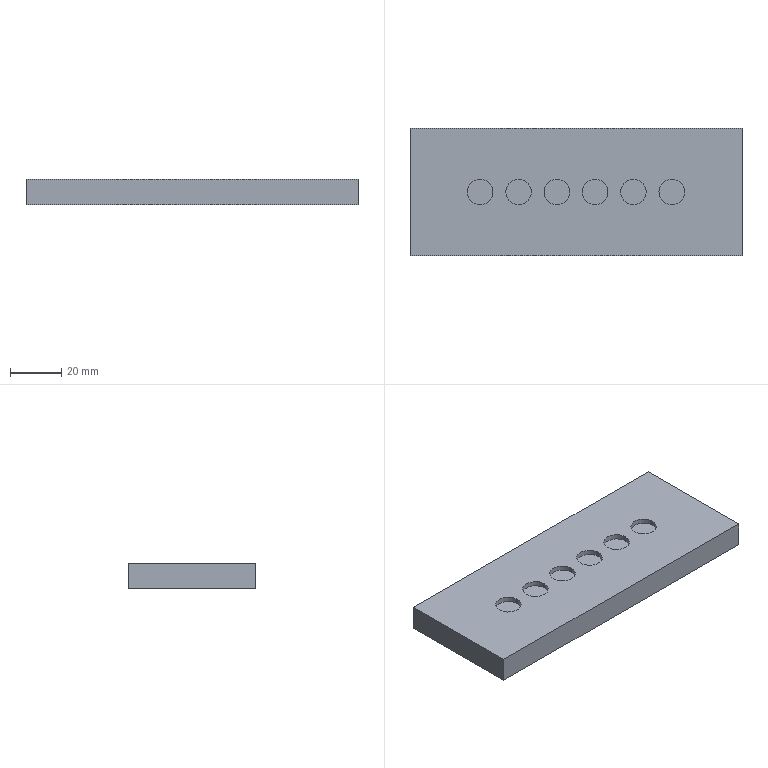Part | SolidWorks | features Extrusion 1, ICE 1 | 1 solid | 24 faces | box 130 x 50 x 10 mm | volume 64058 mm3 | cylinder 12 | plane 12 | commonest cylinder face diameters 10 x12
STEP:
#1=CARTESIAN_POINT('',(-42.5,0.,8.));
#2=VERTEX_POINT('',#1);
#3=CARTESIAN_POINT('',(-32.5,0.,8.));
#4=VERTEX_POINT('',#3);
#5=CARTESIAN_POINT('',(-37.5,0.,8.));
#6=DIRECTION('',(0.,0.,1.));
#7=DIRECTION('',(1.,0.,0.));
#8=AXIS2_PLACEMENT_3D('',#5,#6,#7);
#9=CIRCLE('',#8,5.);
#10=EDGE_CURVE('',#2,#4,#9,.T.);
#11=ORIENTED_EDGE('',*,*,#10,.F.);
#12=CARTESIAN_POINT('',(-42.5,0.,10.));
#13=VERTEX_POINT('',#12);
#14=CARTESIAN_POINT('',(-42.5,0.,8.));
#15=DIRECTION('',(0.,0.,1.));
#16=VECTOR('',#15,1000.);
#17=LINE('',#14,#16);
#18=EDGE_CURVE('',#2,#13,#17,.T.);
#19=ORIENTED_EDGE('',*,*,#18,.T.);
#20=CARTESIAN_POINT('',(-32.5,0.,10.));
#21=VERTEX_POINT('',#20);
#22=CARTESIAN_POINT('',(-37.5,0.,10.));
#23=DIRECTION('',(0.,0.,1.));
#24=DIRECTION('',(1.,0.,0.));
#25=AXIS2_PLACEMENT_3D('',#22,#23,#24);
#26=CIRCLE('',#25,5.);
#27=EDGE_CURVE('',#13,#21,#26,.T.);
#28=ORIENTED_EDGE('',*,*,#27,.T.);
#29=CARTESIAN_POINT('',(-32.5,0.,8.));
#30=DIRECTION('',(0.,0.,1.));
#31=VECTOR('',#30,1000.);
#32=LINE('',#29,#31);
#33=EDGE_CURVE('',#4,#21,#32,.T.);
#34=ORIENTED_EDGE('',*,*,#33,.F.);
#35=EDGE_LOOP('',(#11,#19,#28,#34));
#36=FACE_OUTER_BOUND('',#35,.T.);
#37=CARTESIAN_POINT('',(-37.5,0.,8.));
#38=DIRECTION('',(0.,0.,1.));
#39=DIRECTION('',(1.,0.,0.));
#40=AXIS2_PLACEMENT_3D('',#37,#38,#39);
#41=CYLINDRICAL_SURFACE('',#40,5.);
#42=ADVANCED_FACE('',(#36),#41,.F.);
#43=CARTESIAN_POINT('',(-27.5,0.,8.));
#44=VERTEX_POINT('',#43);
#45=CARTESIAN_POINT('',(-17.5,0.,8.));
#46=VERTEX_POINT('',#45);
#47=CARTESIAN_POINT('',(-22.5,0.,8.));
#48=DIRECTION('',(0.,0.,1.));
#49=DIRECTION('',(1.,0.,0.));
#50=AXIS2_PLACEMENT_3D('',#47,#48,#49);
#51=CIRCLE('',#50,5.);
#52=EDGE_CURVE('',#44,#46,#51,.T.);
#53=ORIENTED_EDGE('',*,*,#52,.F.);
#54=CARTESIAN_POINT('',(-27.5,0.,10.));
#55=VERTEX_POINT('',#54);
#56=CARTESIAN_POINT('',(-27.5,0.,8.));
#57=DIRECTION('',(0.,0.,1.));
#58=VECTOR('',#57,1000.);
#59=LINE('',#56,#58);
#60=EDGE_CURVE('',#44,#55,#59,.T.);
#61=ORIENTED_EDGE('',*,*,#60,.T.);
#62=CARTESIAN_POINT('',(-17.5,0.,10.));
#63=VERTEX_POINT('',#62);
#64=CARTESIAN_POINT('',(-22.5,0.,10.));
#65=DIRECTION('',(0.,0.,1.));
#66=DIRECTION('',(1.,0.,0.));
#67=AXIS2_PLACEMENT_3D('',#64,#65,#66);
#68=CIRCLE('',#67,5.);
#69=EDGE_CURVE('',#55,#63,#68,.T.);
#70=ORIENTED_EDGE('',*,*,#69,.T.);
#71=CARTESIAN_POINT('',(-17.5,0.,8.));
#72=DIRECTION('',(0.,0.,1.));
#73=VECTOR('',#72,1000.);
#74=LINE('',#71,#73);
#75=EDGE_CURVE('',#46,#63,#74,.T.);
#76=ORIENTED_EDGE('',*,*,#75,.F.);
#77=EDGE_LOOP('',(#53,#61,#70,#76));
#78=FACE_OUTER_BOUND('',#77,.T.);
#79=CARTESIAN_POINT('',(-22.5,0.,8.));
#80=DIRECTION('',(0.,0.,1.));
#81=DIRECTION('',(1.,0.,0.));
#82=AXIS2_PLACEMENT_3D('',#79,#80,#81);
#83=CYLINDRICAL_SURFACE('',#82,5.);
#84=ADVANCED_FACE('',(#78),#83,.F.);
#85=CARTESIAN_POINT('',(-12.5,0.,8.));
#86=VERTEX_POINT('',#85);
#87=CARTESIAN_POINT('',(-2.5,0.,8.));
#88=VERTEX_POINT('',#87);
#89=CARTESIAN_POINT('',(-7.5,0.,8.));
#90=DIRECTION('',(0.,0.,1.));
#91=DIRECTION('',(1.,0.,0.));
#92=AXIS2_PLACEMENT_3D('',#89,#90,#91);
#93=CIRCLE('',#92,5.);
#94=EDGE_CURVE('',#86,#88,#93,.T.);
#95=ORIENTED_EDGE('',*,*,#94,.F.);
#96=CARTESIAN_POINT('',(-12.5,0.,10.));
#97=VERTEX_POINT('',#96);
#98=CARTESIAN_POINT('',(-12.5,0.,8.));
#99=DIRECTION('',(0.,0.,1.));
#100=VECTOR('',#99,1000.);
#101=LINE('',#98,#100);
#102=EDGE_CURVE('',#86,#97,#101,.T.);
#103=ORIENTED_EDGE('',*,*,#102,.T.);
#104=CARTESIAN_POINT('',(-2.5,0.,10.));
#105=VERTEX_POINT('',#104);
#106=CARTESIAN_POINT('',(-7.5,0.,10.));
#107=DIRECTION('',(0.,0.,1.));
#108=DIRECTION('',(1.,0.,0.));
#109=AXIS2_PLACEMENT_3D('',#106,#107,#108);
#110=CIRCLE('',#109,5.);
#111=EDGE_CURVE('',#97,#105,#110,.T.);
#112=ORIENTED_EDGE('',*,*,#111,.T.);
#113=CARTESIAN_POINT('',(-2.5,0.,8.));
#114=DIRECTION('',(0.,0.,1.));
#115=VECTOR('',#114,1000.);
#116=LINE('',#113,#115);
#117=EDGE_CURVE('',#88,#105,#116,.T.);
#118=ORIENTED_EDGE('',*,*,#117,.F.);
#119=EDGE_LOOP('',(#95,#103,#112,#118));
#120=FACE_OUTER_BOUND('',#119,.T.);
#121=CARTESIAN_POINT('',(-7.5,0.,8.));
#122=DIRECTION('',(0.,0.,1.));
#123=DIRECTION('',(1.,0.,0.));
#124=AXIS2_PLACEMENT_3D('',#121,#122,#123);
#125=CYLINDRICAL_SURFACE('',#124,5.);
#126=ADVANCED_FACE('',(#120),#125,.F.);
#127=CARTESIAN_POINT('',(2.5,0.,8.));
#128=VERTEX_POINT('',#127);
#129=CARTESIAN_POINT('',(12.5,0.,8.));
#130=VERTEX_POINT('',#129);
#131=CARTESIAN_POINT('',(7.5,0.,8.));
#132=DIRECTION('',(0.,0.,1.));
#133=DIRECTION('',(1.,0.,0.));
#134=AXIS2_PLACEMENT_3D('',#131,#132,#133);
#135=CIRCLE('',#134,5.);
#136=EDGE_CURVE('',#128,#130,#135,.T.);
#137=ORIENTED_EDGE('',*,*,#136,.F.);
#138=CARTESIAN_POINT('',(2.5,0.,10.));
#139=VERTEX_POINT('',#138);
#140=CARTESIAN_POINT('',(2.5,0.,8.));
#141=DIRECTION('',(0.,0.,1.));
#142=VECTOR('',#141,1000.);
#143=LINE('',#140,#142);
#144=EDGE_CURVE('',#128,#139,#143,.T.);
#145=ORIENTED_EDGE('',*,*,#144,.T.);
#146=CARTESIAN_POINT('',(12.5,0.,10.));
#147=VERTEX_POINT('',#146);
#148=CARTESIAN_POINT('',(7.5,0.,10.));
#149=DIRECTION('',(0.,0.,1.));
#150=DIRECTION('',(1.,0.,0.));
#151=AXIS2_PLACEMENT_3D('',#148,#149,#150);
#152=CIRCLE('',#151,5.);
#153=EDGE_CURVE('',#139,#147,#152,.T.);
#154=ORIENTED_EDGE('',*,*,#153,.T.);
#155=CARTESIAN_POINT('',(12.5,0.,8.));
#156=DIRECTION('',(0.,0.,1.));
#157=VECTOR('',#156,1000.);
#158=LINE('',#155,#157);
#159=EDGE_CURVE('',#130,#147,#158,.T.);
#160=ORIENTED_EDGE('',*,*,#159,.F.);
#161=EDGE_LOOP('',(#137,#145,#154,#160));
#162=FACE_OUTER_BOUND('',#161,.T.);
#163=CARTESIAN_POINT('',(7.5,0.,8.));
#164=DIRECTION('',(0.,0.,1.));
#165=DIRECTION('',(1.,0.,0.));
#166=AXIS2_PLACEMENT_3D('',#163,#164,#165);
#167=CYLINDRICAL_SURFACE('',#166,5.);
#168=ADVANCED_FACE('',(#162),#167,.F.);
#169=CARTESIAN_POINT('',(17.5,0.,8.));
#170=VERTEX_POINT('',#169);
#171=CARTESIAN_POINT('',(27.5,0.,8.));
#172=VERTEX_POINT('',#171);
#173=CARTESIAN_POINT('',(22.5,0.,8.));
#174=DIRECTION('',(0.,0.,1.));
#175=DIRECTION('',(1.,0.,0.));
#176=AXIS2_PLACEMENT_3D('',#173,#174,#175);
#177=CIRCLE('',#176,5.);
#178=EDGE_CURVE('',#170,#172,#177,.T.);
#179=ORIENTED_EDGE('',*,*,#178,.F.);
#180=CARTESIAN_POINT('',(17.5,0.,10.));
#181=VERTEX_POINT('',#180);
#182=CARTESIAN_POINT('',(17.5,0.,8.));
#183=DIRECTION('',(0.,0.,1.));
#184=VECTOR('',#183,1000.);
#185=LINE('',#182,#184);
#186=EDGE_CURVE('',#170,#181,#185,.T.);
#187=ORIENTED_EDGE('',*,*,#186,.T.);
#188=CARTESIAN_POINT('',(27.5,0.,10.));
#189=VERTEX_POINT('',#188);
#190=CARTESIAN_POINT('',(22.5,0.,10.));
#191=DIRECTION('',(0.,0.,1.));
#192=DIRECTION('',(1.,0.,0.));
#193=AXIS2_PLACEMENT_3D('',#190,#191,#192);
#194=CIRCLE('',#193,5.);
#195=EDGE_CURVE('',#181,#189,#194,.T.);
#196=ORIENTED_EDGE('',*,*,#195,.T.);
#197=CARTESIAN_POINT('',(27.5,0.,8.));
#198=DIRECTION('',(0.,0.,1.));
#199=VECTOR('',#198,1000.);
#200=LINE('',#197,#199);
#201=EDGE_CURVE('',#172,#189,#200,.T.);
#202=ORIENTED_EDGE('',*,*,#201,.F.);
#203=EDGE_LOOP('',(#179,#187,#196,#202));
#204=FACE_OUTER_BOUND('',#203,.T.);
#205=CARTESIAN_POINT('',(22.5,0.,8.));
#206=DIRECTION('',(0.,0.,1.));
#207=DIRECTION('',(1.,0.,0.));
#208=AXIS2_PLACEMENT_3D('',#205,#206,#207);
#209=CYLINDRICAL_SURFACE('',#208,5.);
#210=ADVANCED_FACE('',(#204),#209,.F.);
#211=CARTESIAN_POINT('',(32.5,0.,8.));
#212=VERTEX_POINT('',#211);
#213=CARTESIAN_POINT('',(42.5,0.,8.));
#214=VERTEX_POINT('',#213);
#215=CARTESIAN_POINT('',(37.5,0.,8.));
#216=DIRECTION('',(0.,0.,1.));
#217=DIRECTION('',(1.,0.,0.));
#218=AXIS2_PLACEMENT_3D('',#215,#216,#217);
#219=CIRCLE('',#218,5.);
#220=EDGE_CURVE('',#212,#214,#219,.T.);
#221=ORIENTED_EDGE('',*,*,#220,.F.);
#222=CARTESIAN_POINT('',(32.5,0.,10.));
#223=VERTEX_POINT('',#222);
#224=CARTESIAN_POINT('',(32.5,0.,8.));
#225=DIRECTION('',(0.,0.,1.));
#226=VECTOR('',#225,1000.);
#227=LINE('',#224,#226);
#228=EDGE_CURVE('',#212,#223,#227,.T.);
#229=ORIENTED_EDGE('',*,*,#228,.T.);
#230=CARTESIAN_POINT('',(42.5,0.,10.));
#231=VERTEX_POINT('',#230);
#232=CARTESIAN_POINT('',(37.5,0.,10.));
#233=DIRECTION('',(0.,0.,1.));
#234=DIRECTION('',(1.,0.,0.));
#235=AXIS2_PLACEMENT_3D('',#232,#233,#234);
#236=CIRCLE('',#235,5.);
#237=EDGE_CURVE('',#223,#231,#236,.T.);
#238=ORIENTED_EDGE('',*,*,#237,.T.);
#239=CARTESIAN_POINT('',(42.5,0.,8.));
#240=DIRECTION('',(0.,0.,1.));
#241=VECTOR('',#240,1000.);
#242=LINE('',#239,#241);
#243=EDGE_CURVE('',#214,#231,#242,.T.);
#244=ORIENTED_EDGE('',*,*,#243,.F.);
#245=EDGE_LOOP('',(#221,#229,#238,#244));
#246=FACE_OUTER_BOUND('',#245,.T.);
#247=CARTESIAN_POINT('',(37.5,0.,8.));
#248=DIRECTION('',(0.,0.,1.));
#249=DIRECTION('',(1.,0.,0.));
#250=AXIS2_PLACEMENT_3D('',#247,#248,#249);
#251=CYLINDRICAL_SURFACE('',#250,5.);
#252=ADVANCED_FACE('',(#246),#251,.F.);
#253=CARTESIAN_POINT('',(-65.,25.,0.));
#254=VERTEX_POINT('',#253);
#255=CARTESIAN_POINT('',(-65.,-25.,0.));
#256=VERTEX_POINT('',#255);
#257=CARTESIAN_POINT('',(-65.,-25.,0.));
#258=DIRECTION('',(0.,-1.,0.));
#259=VECTOR('',#258,1000.);
#260=LINE('',#257,#259);
#261=EDGE_CURVE('',#254,#256,#260,.T.);
#262=ORIENTED_EDGE('',*,*,#261,.T.);
#263=CARTESIAN_POINT('',(-65.,-25.,10.));
#264=VERTEX_POINT('',#263);
#265=CARTESIAN_POINT('',(-65.,-25.,10.));
#266=DIRECTION('',(0.,0.,-1.));
#267=VECTOR('',#266,1000.);
#268=LINE('',#265,#267);
#269=EDGE_CURVE('',#264,#256,#268,.T.);
#270=ORIENTED_EDGE('',*,*,#269,.F.);
#271=CARTESIAN_POINT('',(-65.,25.,10.));
#272=VERTEX_POINT('',#271);
#273=CARTESIAN_POINT('',(-65.,-25.,10.));
#274=DIRECTION('',(0.,-1.,0.));
#275=VECTOR('',#274,1000.);
#276=LINE('',#273,#275);
#277=EDGE_CURVE('',#272,#264,#276,.T.);
#278=ORIENTED_EDGE('',*,*,#277,.F.);
#279=CARTESIAN_POINT('',(-65.,25.,10.));
#280=DIRECTION('',(0.,0.,-1.));
#281=VECTOR('',#280,1000.);
#282=LINE('',#279,#281);
#283=EDGE_CURVE('',#272,#254,#282,.T.);
#284=ORIENTED_EDGE('',*,*,#283,.T.);
#285=EDGE_LOOP('',(#262,#270,#278,#284));
#286=FACE_OUTER_BOUND('',#285,.T.);
#287=CARTESIAN_POINT('',(-65.,-25.,10.));
#288=DIRECTION('',(1.,0.,0.));
#289=DIRECTION('',(0.,0.,-1.));
#290=AXIS2_PLACEMENT_3D('',#287,#288,#289);
#291=PLANE('',#290);
#292=ADVANCED_FACE('',(#286),#291,.F.);
#293=CARTESIAN_POINT('',(65.,-25.,0.));
#294=VERTEX_POINT('',#293);
#295=CARTESIAN_POINT('',(65.,-25.,0.));
#296=DIRECTION('',(1.,0.,0.));
#297=VECTOR('',#296,1000.);
#298=LINE('',#295,#297);
#299=EDGE_CURVE('',#256,#294,#298,.T.);
#300=ORIENTED_EDGE('',*,*,#299,.T.);
#301=CARTESIAN_POINT('',(65.,-25.,10.));
#302=VERTEX_POINT('',#301);
#303=CARTESIAN_POINT('',(65.,-25.,10.));
#304=DIRECTION('',(0.,0.,-1.));
#305=VECTOR('',#304,1000.);
#306=LINE('',#303,#305);
#307=EDGE_CURVE('',#302,#294,#306,.T.);
#308=ORIENTED_EDGE('',*,*,#307,.F.);
#309=CARTESIAN_POINT('',(65.,-25.,10.));
#310=DIRECTION('',(1.,0.,0.));
#311=VECTOR('',#310,1000.);
#312=LINE('',#309,#311);
#313=EDGE_CURVE('',#264,#302,#312,.T.);
#314=ORIENTED_EDGE('',*,*,#313,.F.);
#315=ORIENTED_EDGE('',*,*,#269,.T.);
#316=EDGE_LOOP('',(#300,#308,#314,#315));
#317=FACE_OUTER_BOUND('',#316,.T.);
#318=CARTESIAN_POINT('',(65.,-25.,10.));
#319=DIRECTION('',(0.,1.,0.));
#320=DIRECTION('',(-1.,0.,0.));
#321=AXIS2_PLACEMENT_3D('',#318,#319,#320);
#322=PLANE('',#321);
#323=ADVANCED_FACE('',(#317),#322,.F.);
#324=CARTESIAN_POINT('',(65.,25.,0.));
#325=VERTEX_POINT('',#324);
#326=CARTESIAN_POINT('',(65.,-25.,0.));
#327=DIRECTION('',(0.,1.,0.));
#328=VECTOR('',#327,1000.);
#329=LINE('',#326,#328);
#330=EDGE_CURVE('',#294,#325,#329,.T.);
#331=ORIENTED_EDGE('',*,*,#330,.T.);
#332=CARTESIAN_POINT('',(65.,25.,10.));
#333=VERTEX_POINT('',#332);
#334=CARTESIAN_POINT('',(65.,25.,10.));
#335=DIRECTION('',(0.,0.,-1.));
#336=VECTOR('',#335,1000.);
#337=LINE('',#334,#336);
#338=EDGE_CURVE('',#333,#325,#337,.T.);
#339=ORIENTED_EDGE('',*,*,#338,.F.);
#340=CARTESIAN_POINT('',(65.,-25.,10.));
#341=DIRECTION('',(0.,1.,0.));
#342=VECTOR('',#341,1000.);
#343=LINE('',#340,#342);
#344=EDGE_CURVE('',#302,#333,#343,.T.);
#345=ORIENTED_EDGE('',*,*,#344,.F.);
#346=ORIENTED_EDGE('',*,*,#307,.T.);
#347=EDGE_LOOP('',(#331,#339,#345,#346));
#348=FACE_OUTER_BOUND('',#347,.T.);
#349=CARTESIAN_POINT('',(65.,-25.,10.));
#350=DIRECTION('',(-1.,0.,0.));
#351=DIRECTION('',(0.,0.,1.));
#352=AXIS2_PLACEMENT_3D('',#349,#350,#351);
#353=PLANE('',#352);
#354=ADVANCED_FACE('',(#348),#353,.F.);
#355=CARTESIAN_POINT('',(65.,25.,0.));
#356=DIRECTION('',(-1.,0.,0.));
#357=VECTOR('',#356,1000.);
#358=LINE('',#355,#357);
#359=EDGE_CURVE('',#325,#254,#358,.T.);
#360=ORIENTED_EDGE('',*,*,#359,.T.);
#361=ORIENTED_EDGE('',*,*,#283,.F.);
#362=CARTESIAN_POINT('',(65.,25.,10.));
#363=DIRECTION('',(-1.,0.,0.));
#364=VECTOR('',#363,1000.);
#365=LINE('',#362,#364);
#366=EDGE_CURVE('',#333,#272,#365,.T.);
#367=ORIENTED_EDGE('',*,*,#366,.F.);
#368=ORIENTED_EDGE('',*,*,#338,.T.);
#369=EDGE_LOOP('',(#360,#361,#367,#368));
#370=FACE_OUTER_BOUND('',#369,.T.);
#371=CARTESIAN_POINT('',(65.,25.,10.));
#372=DIRECTION('',(0.,-1.,0.));
#373=DIRECTION('',(1.,0.,0.));
#374=AXIS2_PLACEMENT_3D('',#371,#372,#373);
#375=PLANE('',#374);
#376=ADVANCED_FACE('',(#370),#375,.F.);
#377=CARTESIAN_POINT('',(-37.5,0.,10.));
#378=DIRECTION('',(0.,0.,1.));
#379=DIRECTION('',(1.,0.,0.));
#380=AXIS2_PLACEMENT_3D('',#377,#378,#379);
#381=CIRCLE('',#380,5.);
#382=EDGE_CURVE('',#21,#13,#381,.T.);
#383=ORIENTED_EDGE('',*,*,#382,.F.);
#384=ORIENTED_EDGE('',*,*,#27,.F.);
#385=EDGE_LOOP('',(#383,#384));
#386=FACE_BOUND('',#385,.T.);
#387=CARTESIAN_POINT('',(-22.5,0.,10.));
#388=DIRECTION('',(0.,0.,1.));
#389=DIRECTION('',(1.,0.,0.));
#390=AXIS2_PLACEMENT_3D('',#387,#388,#389);
#391=CIRCLE('',#390,5.);
#392=EDGE_CURVE('',#63,#55,#391,.T.);
#393=ORIENTED_EDGE('',*,*,#392,.F.);
#394=ORIENTED_EDGE('',*,*,#69,.F.);
#395=EDGE_LOOP('',(#393,#394));
#396=FACE_BOUND('',#395,.T.);
#397=CARTESIAN_POINT('',(-7.5,0.,10.));
#398=DIRECTION('',(0.,0.,1.));
#399=DIRECTION('',(1.,0.,0.));
#400=AXIS2_PLACEMENT_3D('',#397,#398,#399);
#401=CIRCLE('',#400,5.);
#402=EDGE_CURVE('',#105,#97,#401,.T.);
#403=ORIENTED_EDGE('',*,*,#402,.F.);
#404=ORIENTED_EDGE('',*,*,#111,.F.);
#405=EDGE_LOOP('',(#403,#404));
#406=FACE_BOUND('',#405,.T.);
#407=CARTESIAN_POINT('',(7.5,0.,10.));
#408=DIRECTION('',(0.,0.,1.));
#409=DIRECTION('',(1.,0.,0.));
#410=AXIS2_PLACEMENT_3D('',#407,#408,#409);
#411=CIRCLE('',#410,5.);
#412=EDGE_CURVE('',#147,#139,#411,.T.);
#413=ORIENTED_EDGE('',*,*,#412,.F.);
#414=ORIENTED_EDGE('',*,*,#153,.F.);
#415=EDGE_LOOP('',(#413,#414));
#416=FACE_BOUND('',#415,.T.);
#417=CARTESIAN_POINT('',(22.5,0.,10.));
#418=DIRECTION('',(0.,0.,1.));
#419=DIRECTION('',(1.,0.,0.));
#420=AXIS2_PLACEMENT_3D('',#417,#418,#419);
#421=CIRCLE('',#420,5.);
#422=EDGE_CURVE('',#189,#181,#421,.T.);
#423=ORIENTED_EDGE('',*,*,#422,.F.);
#424=ORIENTED_EDGE('',*,*,#195,.F.);
#425=EDGE_LOOP('',(#423,#424));
#426=FACE_BOUND('',#425,.T.);
#427=CARTESIAN_POINT('',(37.5,0.,10.));
#428=DIRECTION('',(0.,0.,1.));
#429=DIRECTION('',(1.,0.,0.));
#430=AXIS2_PLACEMENT_3D('',#427,#428,#429);
#431=CIRCLE('',#430,5.);
#432=EDGE_CURVE('',#231,#223,#431,.T.);
#433=ORIENTED_EDGE('',*,*,#432,.F.);
#434=ORIENTED_EDGE('',*,*,#237,.F.);
#435=EDGE_LOOP('',(#433,#434));
#436=FACE_BOUND('',#435,.T.);
#437=ORIENTED_EDGE('',*,*,#277,.T.);
#438=ORIENTED_EDGE('',*,*,#313,.T.);
#439=ORIENTED_EDGE('',*,*,#344,.T.);
#440=ORIENTED_EDGE('',*,*,#366,.T.);
#441=EDGE_LOOP('',(#437,#438,#439,#440));
#442=FACE_OUTER_BOUND('',#441,.T.);
#443=CARTESIAN_POINT('',(0.,0.,10.));
#444=DIRECTION('',(0.,0.,1.));
#445=DIRECTION('',(1.,0.,0.));
#446=AXIS2_PLACEMENT_3D('',#443,#444,#445);
#447=PLANE('',#446);
#448=ADVANCED_FACE('',(#386,#396,#406,#416,#426,#436,#442),#447,.T.);
#449=ORIENTED_EDGE('',*,*,#261,.F.);
#450=ORIENTED_EDGE('',*,*,#359,.F.);
#451=ORIENTED_EDGE('',*,*,#330,.F.);
#452=ORIENTED_EDGE('',*,*,#299,.F.);
#453=EDGE_LOOP('',(#449,#450,#451,#452));
#454=FACE_OUTER_BOUND('',#453,.T.);
#455=CARTESIAN_POINT('',(0.,0.,0.));
#456=DIRECTION('',(0.,0.,1.));
#457=DIRECTION('',(1.,0.,0.));
#458=AXIS2_PLACEMENT_3D('',#455,#456,#457);
#459=PLANE('',#458);
#460=ADVANCED_FACE('',(#454),#459,.F.);
#461=ORIENTED_EDGE('',*,*,#228,.F.);
#462=CARTESIAN_POINT('',(37.5,0.,8.));
#463=DIRECTION('',(0.,0.,1.));
#464=DIRECTION('',(1.,0.,0.));
#465=AXIS2_PLACEMENT_3D('',#462,#463,#464);
#466=CIRCLE('',#465,5.);
#467=EDGE_CURVE('',#214,#212,#466,.T.);
#468=ORIENTED_EDGE('',*,*,#467,.F.);
#469=ORIENTED_EDGE('',*,*,#243,.T.);
#470=ORIENTED_EDGE('',*,*,#432,.T.);
#471=EDGE_LOOP('',(#461,#468,#469,#470));
#472=FACE_OUTER_BOUND('',#471,.T.);
#473=CARTESIAN_POINT('',(37.5,0.,8.));
#474=DIRECTION('',(0.,0.,1.));
#475=DIRECTION('',(1.,0.,0.));
#476=AXIS2_PLACEMENT_3D('',#473,#474,#475);
#477=CYLINDRICAL_SURFACE('',#476,5.);
#478=ADVANCED_FACE('',(#472),#477,.F.);
#479=ORIENTED_EDGE('',*,*,#467,.T.);
#480=ORIENTED_EDGE('',*,*,#220,.T.);
#481=EDGE_LOOP('',(#479,#480));
#482=FACE_OUTER_BOUND('',#481,.T.);
#483=CARTESIAN_POINT('',(37.5,0.,8.));
#484=DIRECTION('',(0.,0.,1.));
#485=DIRECTION('',(1.,0.,0.));
#486=AXIS2_PLACEMENT_3D('',#483,#484,#485);
#487=PLANE('',#486);
#488=ADVANCED_FACE('',(#482),#487,.T.);
#489=ORIENTED_EDGE('',*,*,#186,.F.);
#490=CARTESIAN_POINT('',(22.5,0.,8.));
#491=DIRECTION('',(0.,0.,1.));
#492=DIRECTION('',(1.,0.,0.));
#493=AXIS2_PLACEMENT_3D('',#490,#491,#492);
#494=CIRCLE('',#493,5.);
#495=EDGE_CURVE('',#172,#170,#494,.T.);
#496=ORIENTED_EDGE('',*,*,#495,.F.);
#497=ORIENTED_EDGE('',*,*,#201,.T.);
#498=ORIENTED_EDGE('',*,*,#422,.T.);
#499=EDGE_LOOP('',(#489,#496,#497,#498));
#500=FACE_OUTER_BOUND('',#499,.T.);
#501=CARTESIAN_POINT('',(22.5,0.,8.));
#502=DIRECTION('',(0.,0.,1.));
#503=DIRECTION('',(1.,0.,0.));
#504=AXIS2_PLACEMENT_3D('',#501,#502,#503);
#505=CYLINDRICAL_SURFACE('',#504,5.);
#506=ADVANCED_FACE('',(#500),#505,.F.);
#507=ORIENTED_EDGE('',*,*,#495,.T.);
#508=ORIENTED_EDGE('',*,*,#178,.T.);
#509=EDGE_LOOP('',(#507,#508));
#510=FACE_OUTER_BOUND('',#509,.T.);
#511=CARTESIAN_POINT('',(22.5,0.,8.));
#512=DIRECTION('',(0.,0.,1.));
#513=DIRECTION('',(1.,0.,0.));
#514=AXIS2_PLACEMENT_3D('',#511,#512,#513);
#515=PLANE('',#514);
#516=ADVANCED_FACE('',(#510),#515,.T.);
#517=ORIENTED_EDGE('',*,*,#144,.F.);
#518=CARTESIAN_POINT('',(7.5,0.,8.));
#519=DIRECTION('',(0.,0.,1.));
#520=DIRECTION('',(1.,0.,0.));
#521=AXIS2_PLACEMENT_3D('',#518,#519,#520);
#522=CIRCLE('',#521,5.);
#523=EDGE_CURVE('',#130,#128,#522,.T.);
#524=ORIENTED_EDGE('',*,*,#523,.F.);
#525=ORIENTED_EDGE('',*,*,#159,.T.);
#526=ORIENTED_EDGE('',*,*,#412,.T.);
#527=EDGE_LOOP('',(#517,#524,#525,#526));
#528=FACE_OUTER_BOUND('',#527,.T.);
#529=CARTESIAN_POINT('',(7.5,0.,8.));
#530=DIRECTION('',(0.,0.,1.));
#531=DIRECTION('',(1.,0.,0.));
#532=AXIS2_PLACEMENT_3D('',#529,#530,#531);
#533=CYLINDRICAL_SURFACE('',#532,5.);
#534=ADVANCED_FACE('',(#528),#533,.F.);
#535=ORIENTED_EDGE('',*,*,#523,.T.);
#536=ORIENTED_EDGE('',*,*,#136,.T.);
#537=EDGE_LOOP('',(#535,#536));
#538=FACE_OUTER_BOUND('',#537,.T.);
#539=CARTESIAN_POINT('',(7.5,0.,8.));
#540=DIRECTION('',(0.,0.,1.));
#541=DIRECTION('',(1.,0.,0.));
#542=AXIS2_PLACEMENT_3D('',#539,#540,#541);
#543=PLANE('',#542);
#544=ADVANCED_FACE('',(#538),#543,.T.);
#545=ORIENTED_EDGE('',*,*,#102,.F.);
#546=CARTESIAN_POINT('',(-7.5,0.,8.));
#547=DIRECTION('',(0.,0.,1.));
#548=DIRECTION('',(1.,0.,0.));
#549=AXIS2_PLACEMENT_3D('',#546,#547,#548);
#550=CIRCLE('',#549,5.);
#551=EDGE_CURVE('',#88,#86,#550,.T.);
#552=ORIENTED_EDGE('',*,*,#551,.F.);
#553=ORIENTED_EDGE('',*,*,#117,.T.);
#554=ORIENTED_EDGE('',*,*,#402,.T.);
#555=EDGE_LOOP('',(#545,#552,#553,#554));
#556=FACE_OUTER_BOUND('',#555,.T.);
#557=CARTESIAN_POINT('',(-7.5,0.,8.));
#558=DIRECTION('',(0.,0.,1.));
#559=DIRECTION('',(1.,0.,0.));
#560=AXIS2_PLACEMENT_3D('',#557,#558,#559);
#561=CYLINDRICAL_SURFACE('',#560,5.);
#562=ADVANCED_FACE('',(#556),#561,.F.);
#563=ORIENTED_EDGE('',*,*,#551,.T.);
#564=ORIENTED_EDGE('',*,*,#94,.T.);
#565=EDGE_LOOP('',(#563,#564));
#566=FACE_OUTER_BOUND('',#565,.T.);
#567=CARTESIAN_POINT('',(-7.5,0.,8.));
#568=DIRECTION('',(0.,0.,1.));
#569=DIRECTION('',(1.,0.,0.));
#570=AXIS2_PLACEMENT_3D('',#567,#568,#569);
#571=PLANE('',#570);
#572=ADVANCED_FACE('',(#566),#571,.T.);
#573=ORIENTED_EDGE('',*,*,#60,.F.);
#574=CARTESIAN_POINT('',(-22.5,0.,8.));
#575=DIRECTION('',(0.,0.,1.));
#576=DIRECTION('',(1.,0.,0.));
#577=AXIS2_PLACEMENT_3D('',#574,#575,#576);
#578=CIRCLE('',#577,5.);
#579=EDGE_CURVE('',#46,#44,#578,.T.);
#580=ORIENTED_EDGE('',*,*,#579,.F.);
#581=ORIENTED_EDGE('',*,*,#75,.T.);
#582=ORIENTED_EDGE('',*,*,#392,.T.);
#583=EDGE_LOOP('',(#573,#580,#581,#582));
#584=FACE_OUTER_BOUND('',#583,.T.);
#585=CARTESIAN_POINT('',(-22.5,0.,8.));
#586=DIRECTION('',(0.,0.,1.));
#587=DIRECTION('',(1.,0.,0.));
#588=AXIS2_PLACEMENT_3D('',#585,#586,#587);
#589=CYLINDRICAL_SURFACE('',#588,5.);
#590=ADVANCED_FACE('',(#584),#589,.F.);
#591=ORIENTED_EDGE('',*,*,#579,.T.);
#592=ORIENTED_EDGE('',*,*,#52,.T.);
#593=EDGE_LOOP('',(#591,#592));
#594=FACE_OUTER_BOUND('',#593,.T.);
#595=CARTESIAN_POINT('',(-22.5,0.,8.));
#596=DIRECTION('',(0.,0.,1.));
#597=DIRECTION('',(1.,0.,0.));
#598=AXIS2_PLACEMENT_3D('',#595,#596,#597);
#599=PLANE('',#598);
#600=ADVANCED_FACE('',(#594),#599,.T.);
#601=ORIENTED_EDGE('',*,*,#18,.F.);
#602=CARTESIAN_POINT('',(-37.5,0.,8.));
#603=DIRECTION('',(0.,0.,1.));
#604=DIRECTION('',(1.,0.,0.));
#605=AXIS2_PLACEMENT_3D('',#602,#603,#604);
#606=CIRCLE('',#605,5.);
#607=EDGE_CURVE('',#4,#2,#606,.T.);
#608=ORIENTED_EDGE('',*,*,#607,.F.);
#609=ORIENTED_EDGE('',*,*,#33,.T.);
#610=ORIENTED_EDGE('',*,*,#382,.T.);
#611=EDGE_LOOP('',(#601,#608,#609,#610));
#612=FACE_OUTER_BOUND('',#611,.T.);
#613=CARTESIAN_POINT('',(-37.5,0.,8.));
#614=DIRECTION('',(0.,0.,1.));
#615=DIRECTION('',(1.,0.,0.));
#616=AXIS2_PLACEMENT_3D('',#613,#614,#615);
#617=CYLINDRICAL_SURFACE('',#616,5.);
#618=ADVANCED_FACE('',(#612),#617,.F.);
#619=ORIENTED_EDGE('',*,*,#607,.T.);
#620=ORIENTED_EDGE('',*,*,#10,.T.);
#621=EDGE_LOOP('',(#619,#620));
#622=FACE_OUTER_BOUND('',#621,.T.);
#623=CARTESIAN_POINT('',(-37.5,0.,8.));
#624=DIRECTION('',(0.,0.,1.));
#625=DIRECTION('',(1.,0.,0.));
#626=AXIS2_PLACEMENT_3D('',#623,#624,#625);
#627=PLANE('',#626);
#628=ADVANCED_FACE('',(#622),#627,.T.);
#629=CLOSED_SHELL('',(#42,#84,#126,#168,#210,#252,#292,#323,#354,#376,#448,#460,#478,#488,#506,#516,#534,#544,#562,#572,#590,#600,#618,#628));
#630=MANIFOLD_SOLID_BREP('',#629);
#631=CARTESIAN_POINT('',(0.,0.,0.));
#632=DIRECTION('',(0.,0.,1.));
#633=DIRECTION('',(1.,0.,0.));
#634=AXIS2_PLACEMENT_3D('',#631,#632,#633);
#635=(LENGTH_UNIT()NAMED_UNIT(*)SI_UNIT(.MILLI.,.METRE.));
#636=UNCERTAINTY_MEASURE_WITH_UNIT(LENGTH_MEASURE(0.00001),#635,'','');
#637=(NAMED_UNIT(*)PLANE_ANGLE_UNIT()SI_UNIT($,.RADIAN.));
#638=(NAMED_UNIT(*)SI_UNIT($,.STERADIAN.)SOLID_ANGLE_UNIT());
#639=(GEOMETRIC_REPRESENTATION_CONTEXT(3)GLOBAL_UNCERTAINTY_ASSIGNED_CONTEXT((#636))GLOBAL_UNIT_ASSIGNED_CONTEXT((#635,#637,#638))REPRESENTATION_CONTEXT('',''));
#640=ADVANCED_BREP_SHAPE_REPRESENTATION('',(#630,#634),#639);